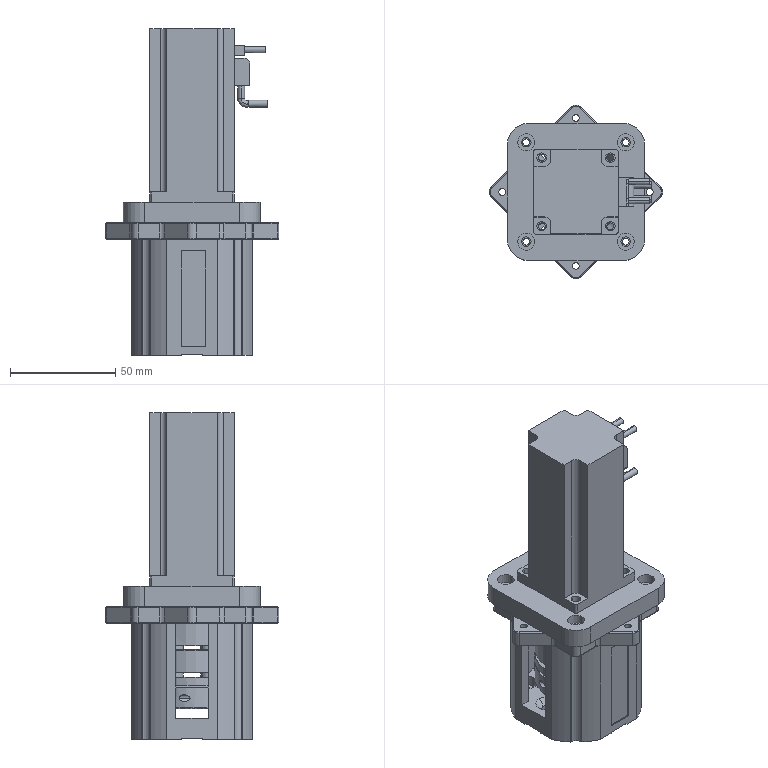Part | STEP file | Copy of 100W motor assembly (universal motor base)^K50A-1H20-S(formula driven)-L300-motor left- | 5 solids | 532 faces | box 82.368 x 82.368 x 154.9 mm | volume 253997 mm3 | cylinder 301 | plane 158 | torus 50 | cone 17 | spline 6 | commonest cylinder face diameters 8 x52 1 x40 6 x32 7 x28 4.5 x20 3.2 x16